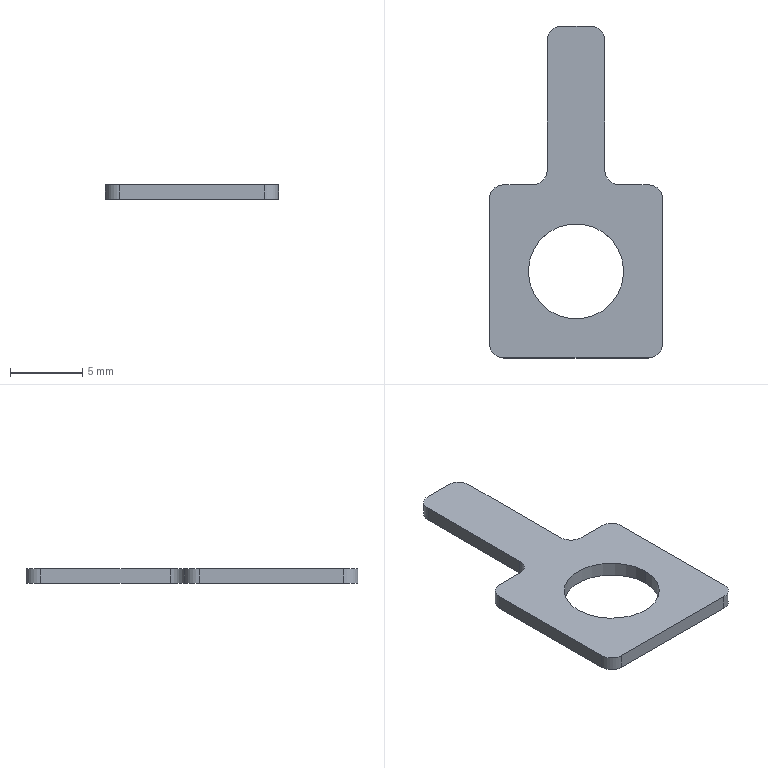Part | SolidWorks | features Extrusion 1, Fillet 1, HoleWzd 1 | 1 solid | 20 faces | box 12 x 23 x 1 mm | volume 152.93 mm3 | cylinder 10 | plane 10 | commonest cylinder face diameters 2 x8 6.6 x2
STEP:
#1=CARTESIAN_POINT('',(-3.3,0.,0.));
#2=VERTEX_POINT('',#1);
#3=CARTESIAN_POINT('',(3.3,0.,0.));
#4=VERTEX_POINT('',#3);
#5=CARTESIAN_POINT('',(0.,0.,0.));
#6=DIRECTION('',(0.,0.,1.));
#7=DIRECTION('',(1.,0.,0.));
#8=AXIS2_PLACEMENT_3D('',#5,#6,#7);
#9=CIRCLE('',#8,3.3);
#10=EDGE_CURVE('',#2,#4,#9,.T.);
#11=ORIENTED_EDGE('',*,*,#10,.F.);
#12=CARTESIAN_POINT('',(-3.3,0.,1.));
#13=VERTEX_POINT('',#12);
#14=CARTESIAN_POINT('',(-3.3,0.,1.));
#15=DIRECTION('',(0.,0.,1.));
#16=VECTOR('',#15,1000.);
#17=LINE('',#14,#16);
#18=EDGE_CURVE('',#2,#13,#17,.T.);
#19=ORIENTED_EDGE('',*,*,#18,.T.);
#20=CARTESIAN_POINT('',(3.3,0.,1.));
#21=VERTEX_POINT('',#20);
#22=CARTESIAN_POINT('',(0.,0.,1.));
#23=DIRECTION('',(0.,0.,1.));
#24=DIRECTION('',(1.,0.,0.));
#25=AXIS2_PLACEMENT_3D('',#22,#23,#24);
#26=CIRCLE('',#25,3.3);
#27=EDGE_CURVE('',#13,#21,#26,.T.);
#28=ORIENTED_EDGE('',*,*,#27,.T.);
#29=CARTESIAN_POINT('',(3.3,0.,1.));
#30=DIRECTION('',(0.,0.,1.));
#31=VECTOR('',#30,1000.);
#32=LINE('',#29,#31);
#33=EDGE_CURVE('',#4,#21,#32,.T.);
#34=ORIENTED_EDGE('',*,*,#33,.F.);
#35=EDGE_LOOP('',(#11,#19,#28,#34));
#36=FACE_OUTER_BOUND('',#35,.T.);
#37=CARTESIAN_POINT('',(0.,0.,1.));
#38=DIRECTION('',(0.,0.,1.));
#39=DIRECTION('',(1.,0.,0.));
#40=AXIS2_PLACEMENT_3D('',#37,#38,#39);
#41=CYLINDRICAL_SURFACE('',#40,3.3);
#42=ADVANCED_FACE('',(#36),#41,.F.);
#43=CARTESIAN_POINT('',(6.,-5.,1.));
#44=VERTEX_POINT('',#43);
#45=CARTESIAN_POINT('',(6.,5.,1.));
#46=VERTEX_POINT('',#45);
#47=CARTESIAN_POINT('',(6.,6.,1.));
#48=DIRECTION('',(0.,1.,0.));
#49=VECTOR('',#48,1000.);
#50=LINE('',#47,#49);
#51=EDGE_CURVE('',#44,#46,#50,.T.);
#52=ORIENTED_EDGE('',*,*,#51,.F.);
#53=CARTESIAN_POINT('',(6.,-5.,0.));
#54=VERTEX_POINT('',#53);
#55=CARTESIAN_POINT('',(6.,-5.,1.));
#56=DIRECTION('',(0.,0.,-1.));
#57=VECTOR('',#56,1000.);
#58=LINE('',#55,#57);
#59=EDGE_CURVE('',#44,#54,#58,.T.);
#60=ORIENTED_EDGE('',*,*,#59,.T.);
#61=CARTESIAN_POINT('',(6.,5.,0.));
#62=VERTEX_POINT('',#61);
#63=CARTESIAN_POINT('',(6.,6.,0.));
#64=DIRECTION('',(0.,1.,0.));
#65=VECTOR('',#64,1000.);
#66=LINE('',#63,#65);
#67=EDGE_CURVE('',#54,#62,#66,.T.);
#68=ORIENTED_EDGE('',*,*,#67,.T.);
#69=CARTESIAN_POINT('',(6.,5.,1.));
#70=DIRECTION('',(0.,0.,1.));
#71=VECTOR('',#70,1000.);
#72=LINE('',#69,#71);
#73=EDGE_CURVE('',#62,#46,#72,.T.);
#74=ORIENTED_EDGE('',*,*,#73,.T.);
#75=EDGE_LOOP('',(#52,#60,#68,#74));
#76=FACE_OUTER_BOUND('',#75,.T.);
#77=CARTESIAN_POINT('',(6.,6.,1.));
#78=DIRECTION('',(-1.,0.,0.));
#79=DIRECTION('',(0.,-1.,0.));
#80=AXIS2_PLACEMENT_3D('',#77,#78,#79);
#81=PLANE('',#80);
#82=ADVANCED_FACE('',(#76),#81,.F.);
#83=CARTESIAN_POINT('',(5.,6.,1.));
#84=VERTEX_POINT('',#83);
#85=CARTESIAN_POINT('',(3.,6.,1.));
#86=VERTEX_POINT('',#85);
#87=CARTESIAN_POINT('',(2.,6.,1.));
#88=DIRECTION('',(-1.,0.,0.));
#89=VECTOR('',#88,1000.);
#90=LINE('',#87,#89);
#91=EDGE_CURVE('',#84,#86,#90,.T.);
#92=ORIENTED_EDGE('',*,*,#91,.F.);
#93=CARTESIAN_POINT('',(5.,6.,0.));
#94=VERTEX_POINT('',#93);
#95=CARTESIAN_POINT('',(5.,6.,1.));
#96=DIRECTION('',(0.,0.,-1.));
#97=VECTOR('',#96,1000.);
#98=LINE('',#95,#97);
#99=EDGE_CURVE('',#84,#94,#98,.T.);
#100=ORIENTED_EDGE('',*,*,#99,.T.);
#101=CARTESIAN_POINT('',(3.,6.,0.));
#102=VERTEX_POINT('',#101);
#103=CARTESIAN_POINT('',(2.,6.,0.));
#104=DIRECTION('',(-1.,0.,0.));
#105=VECTOR('',#104,1000.);
#106=LINE('',#103,#105);
#107=EDGE_CURVE('',#94,#102,#106,.T.);
#108=ORIENTED_EDGE('',*,*,#107,.T.);
#109=CARTESIAN_POINT('',(3.,6.,1.));
#110=DIRECTION('',(0.,0.,1.));
#111=VECTOR('',#110,1000.);
#112=LINE('',#109,#111);
#113=EDGE_CURVE('',#102,#86,#112,.T.);
#114=ORIENTED_EDGE('',*,*,#113,.T.);
#115=EDGE_LOOP('',(#92,#100,#108,#114));
#116=FACE_OUTER_BOUND('',#115,.T.);
#117=CARTESIAN_POINT('',(2.,6.,1.));
#118=DIRECTION('',(0.,-1.,0.));
#119=DIRECTION('',(1.,0.,0.));
#120=AXIS2_PLACEMENT_3D('',#117,#118,#119);
#121=PLANE('',#120);
#122=ADVANCED_FACE('',(#116),#121,.F.);
#123=CARTESIAN_POINT('',(2.,7.,1.));
#124=VERTEX_POINT('',#123);
#125=CARTESIAN_POINT('',(2.,16.,1.));
#126=VERTEX_POINT('',#125);
#127=CARTESIAN_POINT('',(2.,6.,1.));
#128=DIRECTION('',(0.,1.,0.));
#129=VECTOR('',#128,1000.);
#130=LINE('',#127,#129);
#131=EDGE_CURVE('',#124,#126,#130,.T.);
#132=ORIENTED_EDGE('',*,*,#131,.F.);
#133=CARTESIAN_POINT('',(2.,7.,0.));
#134=VERTEX_POINT('',#133);
#135=CARTESIAN_POINT('',(2.,7.,0.));
#136=DIRECTION('',(0.,0.,-1.));
#137=VECTOR('',#136,1000.);
#138=LINE('',#135,#137);
#139=EDGE_CURVE('',#124,#134,#138,.T.);
#140=ORIENTED_EDGE('',*,*,#139,.T.);
#141=CARTESIAN_POINT('',(2.,16.,0.));
#142=VERTEX_POINT('',#141);
#143=CARTESIAN_POINT('',(2.,6.,0.));
#144=DIRECTION('',(0.,1.,0.));
#145=VECTOR('',#144,1000.);
#146=LINE('',#143,#145);
#147=EDGE_CURVE('',#134,#142,#146,.T.);
#148=ORIENTED_EDGE('',*,*,#147,.T.);
#149=CARTESIAN_POINT('',(2.,16.,1.));
#150=DIRECTION('',(0.,0.,1.));
#151=VECTOR('',#150,1000.);
#152=LINE('',#149,#151);
#153=EDGE_CURVE('',#142,#126,#152,.T.);
#154=ORIENTED_EDGE('',*,*,#153,.T.);
#155=EDGE_LOOP('',(#132,#140,#148,#154));
#156=FACE_OUTER_BOUND('',#155,.T.);
#157=CARTESIAN_POINT('',(2.,6.,1.));
#158=DIRECTION('',(-1.,0.,0.));
#159=DIRECTION('',(0.,-1.,0.));
#160=AXIS2_PLACEMENT_3D('',#157,#158,#159);
#161=PLANE('',#160);
#162=ADVANCED_FACE('',(#156),#161,.F.);
#163=CARTESIAN_POINT('',(1.,17.,0.));
#164=VERTEX_POINT('',#163);
#165=CARTESIAN_POINT('',(-1.,17.,0.));
#166=VERTEX_POINT('',#165);
#167=CARTESIAN_POINT('',(-2.,17.,0.));
#168=DIRECTION('',(-1.,0.,0.));
#169=VECTOR('',#168,1000.);
#170=LINE('',#167,#169);
#171=EDGE_CURVE('',#164,#166,#170,.T.);
#172=ORIENTED_EDGE('',*,*,#171,.T.);
#173=CARTESIAN_POINT('',(-1.,17.,1.));
#174=VERTEX_POINT('',#173);
#175=CARTESIAN_POINT('',(-1.,17.,1.));
#176=DIRECTION('',(0.,0.,1.));
#177=VECTOR('',#176,1000.);
#178=LINE('',#175,#177);
#179=EDGE_CURVE('',#166,#174,#178,.T.);
#180=ORIENTED_EDGE('',*,*,#179,.T.);
#181=CARTESIAN_POINT('',(1.,17.,1.));
#182=VERTEX_POINT('',#181);
#183=CARTESIAN_POINT('',(-2.,17.,1.));
#184=DIRECTION('',(-1.,0.,0.));
#185=VECTOR('',#184,1000.);
#186=LINE('',#183,#185);
#187=EDGE_CURVE('',#182,#174,#186,.T.);
#188=ORIENTED_EDGE('',*,*,#187,.F.);
#189=CARTESIAN_POINT('',(1.,17.,1.));
#190=DIRECTION('',(0.,0.,-1.));
#191=VECTOR('',#190,1000.);
#192=LINE('',#189,#191);
#193=EDGE_CURVE('',#182,#164,#192,.T.);
#194=ORIENTED_EDGE('',*,*,#193,.T.);
#195=EDGE_LOOP('',(#172,#180,#188,#194));
#196=FACE_OUTER_BOUND('',#195,.T.);
#197=CARTESIAN_POINT('',(-2.,17.,1.));
#198=DIRECTION('',(0.,-1.,0.));
#199=DIRECTION('',(0.,0.,-1.));
#200=AXIS2_PLACEMENT_3D('',#197,#198,#199);
#201=PLANE('',#200);
#202=ADVANCED_FACE('',(#196),#201,.F.);
#203=CARTESIAN_POINT('',(-2.,16.,0.));
#204=VERTEX_POINT('',#203);
#205=CARTESIAN_POINT('',(-2.,7.,0.));
#206=VERTEX_POINT('',#205);
#207=CARTESIAN_POINT('',(-2.,6.,0.));
#208=DIRECTION('',(0.,-1.,0.));
#209=VECTOR('',#208,1000.);
#210=LINE('',#207,#209);
#211=EDGE_CURVE('',#204,#206,#210,.T.);
#212=ORIENTED_EDGE('',*,*,#211,.T.);
#213=CARTESIAN_POINT('',(-2.,7.,1.));
#214=VERTEX_POINT('',#213);
#215=CARTESIAN_POINT('',(-2.,7.,1.));
#216=DIRECTION('',(0.,0.,1.));
#217=VECTOR('',#216,1000.);
#218=LINE('',#215,#217);
#219=EDGE_CURVE('',#206,#214,#218,.T.);
#220=ORIENTED_EDGE('',*,*,#219,.T.);
#221=CARTESIAN_POINT('',(-2.,16.,1.));
#222=VERTEX_POINT('',#221);
#223=CARTESIAN_POINT('',(-2.,6.,1.));
#224=DIRECTION('',(0.,-1.,0.));
#225=VECTOR('',#224,1000.);
#226=LINE('',#223,#225);
#227=EDGE_CURVE('',#222,#214,#226,.T.);
#228=ORIENTED_EDGE('',*,*,#227,.F.);
#229=CARTESIAN_POINT('',(-2.,16.,1.));
#230=DIRECTION('',(0.,0.,-1.));
#231=VECTOR('',#230,1000.);
#232=LINE('',#229,#231);
#233=EDGE_CURVE('',#222,#204,#232,.T.);
#234=ORIENTED_EDGE('',*,*,#233,.T.);
#235=EDGE_LOOP('',(#212,#220,#228,#234));
#236=FACE_OUTER_BOUND('',#235,.T.);
#237=CARTESIAN_POINT('',(-2.,6.,1.));
#238=DIRECTION('',(1.,0.,0.));
#239=DIRECTION('',(0.,0.,-1.));
#240=AXIS2_PLACEMENT_3D('',#237,#238,#239);
#241=PLANE('',#240);
#242=ADVANCED_FACE('',(#236),#241,.F.);
#243=CARTESIAN_POINT('',(-3.,6.,0.));
#244=VERTEX_POINT('',#243);
#245=CARTESIAN_POINT('',(-5.,6.,0.));
#246=VERTEX_POINT('',#245);
#247=CARTESIAN_POINT('',(-6.,6.,0.));
#248=DIRECTION('',(-1.,0.,0.));
#249=VECTOR('',#248,1000.);
#250=LINE('',#247,#249);
#251=EDGE_CURVE('',#244,#246,#250,.T.);
#252=ORIENTED_EDGE('',*,*,#251,.T.);
#253=CARTESIAN_POINT('',(-5.,6.,1.));
#254=VERTEX_POINT('',#253);
#255=CARTESIAN_POINT('',(-5.,6.,1.));
#256=DIRECTION('',(0.,0.,1.));
#257=VECTOR('',#256,1000.);
#258=LINE('',#255,#257);
#259=EDGE_CURVE('',#246,#254,#258,.T.);
#260=ORIENTED_EDGE('',*,*,#259,.T.);
#261=CARTESIAN_POINT('',(-3.,6.,1.));
#262=VERTEX_POINT('',#261);
#263=CARTESIAN_POINT('',(-6.,6.,1.));
#264=DIRECTION('',(-1.,0.,0.));
#265=VECTOR('',#264,1000.);
#266=LINE('',#263,#265);
#267=EDGE_CURVE('',#262,#254,#266,.T.);
#268=ORIENTED_EDGE('',*,*,#267,.F.);
#269=CARTESIAN_POINT('',(-3.,6.,0.));
#270=DIRECTION('',(0.,0.,-1.));
#271=VECTOR('',#270,1000.);
#272=LINE('',#269,#271);
#273=EDGE_CURVE('',#262,#244,#272,.T.);
#274=ORIENTED_EDGE('',*,*,#273,.T.);
#275=EDGE_LOOP('',(#252,#260,#268,#274));
#276=FACE_OUTER_BOUND('',#275,.T.);
#277=CARTESIAN_POINT('',(-6.,6.,1.));
#278=DIRECTION('',(0.,-1.,0.));
#279=DIRECTION('',(1.,0.,0.));
#280=AXIS2_PLACEMENT_3D('',#277,#278,#279);
#281=PLANE('',#280);
#282=ADVANCED_FACE('',(#276),#281,.F.);
#283=CARTESIAN_POINT('',(-6.,5.,1.));
#284=VERTEX_POINT('',#283);
#285=CARTESIAN_POINT('',(-6.,-5.,1.));
#286=VERTEX_POINT('',#285);
#287=CARTESIAN_POINT('',(-6.,6.,1.));
#288=DIRECTION('',(0.,-1.,0.));
#289=VECTOR('',#288,1000.);
#290=LINE('',#287,#289);
#291=EDGE_CURVE('',#284,#286,#290,.T.);
#292=ORIENTED_EDGE('',*,*,#291,.F.);
#293=CARTESIAN_POINT('',(-6.,5.,0.));
#294=VERTEX_POINT('',#293);
#295=CARTESIAN_POINT('',(-6.,5.,1.));
#296=DIRECTION('',(0.,0.,-1.));
#297=VECTOR('',#296,1000.);
#298=LINE('',#295,#297);
#299=EDGE_CURVE('',#284,#294,#298,.T.);
#300=ORIENTED_EDGE('',*,*,#299,.T.);
#301=CARTESIAN_POINT('',(-6.,-5.,0.));
#302=VERTEX_POINT('',#301);
#303=CARTESIAN_POINT('',(-6.,6.,0.));
#304=DIRECTION('',(0.,-1.,0.));
#305=VECTOR('',#304,1000.);
#306=LINE('',#303,#305);
#307=EDGE_CURVE('',#294,#302,#306,.T.);
#308=ORIENTED_EDGE('',*,*,#307,.T.);
#309=CARTESIAN_POINT('',(-6.,-5.,1.));
#310=DIRECTION('',(0.,0.,1.));
#311=VECTOR('',#310,1000.);
#312=LINE('',#309,#311);
#313=EDGE_CURVE('',#302,#286,#312,.T.);
#314=ORIENTED_EDGE('',*,*,#313,.T.);
#315=EDGE_LOOP('',(#292,#300,#308,#314));
#316=FACE_OUTER_BOUND('',#315,.T.);
#317=CARTESIAN_POINT('',(-6.,6.,1.));
#318=DIRECTION('',(1.,0.,0.));
#319=DIRECTION('',(0.,1.,0.));
#320=AXIS2_PLACEMENT_3D('',#317,#318,#319);
#321=PLANE('',#320);
#322=ADVANCED_FACE('',(#316),#321,.F.);
#323=CARTESIAN_POINT('',(-5.,-6.,1.));
#324=VERTEX_POINT('',#323);
#325=CARTESIAN_POINT('',(5.,-6.,1.));
#326=VERTEX_POINT('',#325);
#327=CARTESIAN_POINT('',(-6.,-6.,1.));
#328=DIRECTION('',(1.,0.,0.));
#329=VECTOR('',#328,1000.);
#330=LINE('',#327,#329);
#331=EDGE_CURVE('',#324,#326,#330,.T.);
#332=ORIENTED_EDGE('',*,*,#331,.F.);
#333=CARTESIAN_POINT('',(-5.,-6.,0.));
#334=VERTEX_POINT('',#333);
#335=CARTESIAN_POINT('',(-5.,-6.,1.));
#336=DIRECTION('',(0.,0.,-1.));
#337=VECTOR('',#336,1000.);
#338=LINE('',#335,#337);
#339=EDGE_CURVE('',#324,#334,#338,.T.);
#340=ORIENTED_EDGE('',*,*,#339,.T.);
#341=CARTESIAN_POINT('',(5.,-6.,0.));
#342=VERTEX_POINT('',#341);
#343=CARTESIAN_POINT('',(-6.,-6.,0.));
#344=DIRECTION('',(1.,0.,0.));
#345=VECTOR('',#344,1000.);
#346=LINE('',#343,#345);
#347=EDGE_CURVE('',#334,#342,#346,.T.);
#348=ORIENTED_EDGE('',*,*,#347,.T.);
#349=CARTESIAN_POINT('',(5.,-6.,1.));
#350=DIRECTION('',(0.,0.,1.));
#351=VECTOR('',#350,1000.);
#352=LINE('',#349,#351);
#353=EDGE_CURVE('',#342,#326,#352,.T.);
#354=ORIENTED_EDGE('',*,*,#353,.T.);
#355=EDGE_LOOP('',(#332,#340,#348,#354));
#356=FACE_OUTER_BOUND('',#355,.T.);
#357=CARTESIAN_POINT('',(-6.,-6.,1.));
#358=DIRECTION('',(0.,1.,0.));
#359=DIRECTION('',(0.,0.,1.));
#360=AXIS2_PLACEMENT_3D('',#357,#358,#359);
#361=PLANE('',#360);
#362=ADVANCED_FACE('',(#356),#361,.F.);
#363=CARTESIAN_POINT('',(0.,0.,1.));
#364=DIRECTION('',(0.,0.,1.));
#365=DIRECTION('',(1.,0.,0.));
#366=AXIS2_PLACEMENT_3D('',#363,#364,#365);
#367=CIRCLE('',#366,3.3);
#368=EDGE_CURVE('',#21,#13,#367,.T.);
#369=ORIENTED_EDGE('',*,*,#368,.F.);
#370=ORIENTED_EDGE('',*,*,#27,.F.);
#371=EDGE_LOOP('',(#369,#370));
#372=FACE_BOUND('',#371,.T.);
#373=ORIENTED_EDGE('',*,*,#267,.T.);
#374=CARTESIAN_POINT('',(-5.,5.,1.));
#375=DIRECTION('',(0.,0.,1.));
#376=DIRECTION('',(1.,0.,0.));
#377=AXIS2_PLACEMENT_3D('',#374,#375,#376);
#378=CIRCLE('',#377,1.);
#379=EDGE_CURVE('',#254,#284,#378,.T.);
#380=ORIENTED_EDGE('',*,*,#379,.T.);
#381=ORIENTED_EDGE('',*,*,#291,.T.);
#382=CARTESIAN_POINT('',(-5.,-5.,1.));
#383=DIRECTION('',(0.,0.,1.));
#384=DIRECTION('',(1.,0.,0.));
#385=AXIS2_PLACEMENT_3D('',#382,#383,#384);
#386=CIRCLE('',#385,1.);
#387=EDGE_CURVE('',#286,#324,#386,.T.);
#388=ORIENTED_EDGE('',*,*,#387,.T.);
#389=ORIENTED_EDGE('',*,*,#331,.T.);
#390=CARTESIAN_POINT('',(5.,-5.,1.));
#391=DIRECTION('',(0.,0.,1.));
#392=DIRECTION('',(1.,0.,0.));
#393=AXIS2_PLACEMENT_3D('',#390,#391,#392);
#394=CIRCLE('',#393,1.);
#395=EDGE_CURVE('',#326,#44,#394,.T.);
#396=ORIENTED_EDGE('',*,*,#395,.T.);
#397=ORIENTED_EDGE('',*,*,#51,.T.);
#398=CARTESIAN_POINT('',(5.,5.,1.));
#399=DIRECTION('',(0.,0.,1.));
#400=DIRECTION('',(1.,0.,0.));
#401=AXIS2_PLACEMENT_3D('',#398,#399,#400);
#402=CIRCLE('',#401,1.);
#403=EDGE_CURVE('',#46,#84,#402,.T.);
#404=ORIENTED_EDGE('',*,*,#403,.T.);
#405=ORIENTED_EDGE('',*,*,#91,.T.);
#406=CARTESIAN_POINT('',(3.,7.,1.));
#407=DIRECTION('',(0.,0.,-1.));
#408=DIRECTION('',(1.,0.,0.));
#409=AXIS2_PLACEMENT_3D('',#406,#407,#408);
#410=CIRCLE('',#409,1.);
#411=EDGE_CURVE('',#86,#124,#410,.T.);
#412=ORIENTED_EDGE('',*,*,#411,.T.);
#413=ORIENTED_EDGE('',*,*,#131,.T.);
#414=CARTESIAN_POINT('',(1.,16.,1.));
#415=DIRECTION('',(0.,0.,1.));
#416=DIRECTION('',(1.,0.,0.));
#417=AXIS2_PLACEMENT_3D('',#414,#415,#416);
#418=CIRCLE('',#417,1.);
#419=EDGE_CURVE('',#126,#182,#418,.T.);
#420=ORIENTED_EDGE('',*,*,#419,.T.);
#421=ORIENTED_EDGE('',*,*,#187,.T.);
#422=CARTESIAN_POINT('',(-1.,16.,1.));
#423=DIRECTION('',(0.,0.,1.));
#424=DIRECTION('',(1.,0.,0.));
#425=AXIS2_PLACEMENT_3D('',#422,#423,#424);
#426=CIRCLE('',#425,1.);
#427=EDGE_CURVE('',#174,#222,#426,.T.);
#428=ORIENTED_EDGE('',*,*,#427,.T.);
#429=ORIENTED_EDGE('',*,*,#227,.T.);
#430=CARTESIAN_POINT('',(-3.,7.,1.));
#431=DIRECTION('',(0.,0.,-1.));
#432=DIRECTION('',(1.,0.,0.));
#433=AXIS2_PLACEMENT_3D('',#430,#431,#432);
#434=CIRCLE('',#433,1.);
#435=EDGE_CURVE('',#214,#262,#434,.T.);
#436=ORIENTED_EDGE('',*,*,#435,.T.);
#437=EDGE_LOOP('',(#373,#380,#381,#388,#389,#396,#397,#404,#405,#412,#413,#420,#421,#428,#429,#436));
#438=FACE_OUTER_BOUND('',#437,.T.);
#439=CARTESIAN_POINT('',(0.,0.,1.));
#440=DIRECTION('',(0.,0.,1.));
#441=DIRECTION('',(1.,0.,0.));
#442=AXIS2_PLACEMENT_3D('',#439,#440,#441);
#443=PLANE('',#442);
#444=ADVANCED_FACE('',(#372,#438),#443,.T.);
#445=CARTESIAN_POINT('',(0.,0.,0.));
#446=DIRECTION('',(0.,0.,1.));
#447=DIRECTION('',(1.,0.,0.));
#448=AXIS2_PLACEMENT_3D('',#445,#446,#447);
#449=CIRCLE('',#448,3.3);
#450=EDGE_CURVE('',#4,#2,#449,.T.);
#451=ORIENTED_EDGE('',*,*,#450,.T.);
#452=ORIENTED_EDGE('',*,*,#10,.T.);
#453=EDGE_LOOP('',(#451,#452));
#454=FACE_BOUND('',#453,.T.);
#455=ORIENTED_EDGE('',*,*,#307,.F.);
#456=CARTESIAN_POINT('',(-5.,5.,0.));
#457=DIRECTION('',(0.,0.,-1.));
#458=DIRECTION('',(1.,0.,0.));
#459=AXIS2_PLACEMENT_3D('',#456,#457,#458);
#460=CIRCLE('',#459,1.);
#461=EDGE_CURVE('',#294,#246,#460,.T.);
#462=ORIENTED_EDGE('',*,*,#461,.T.);
#463=ORIENTED_EDGE('',*,*,#251,.F.);
#464=CARTESIAN_POINT('',(-3.,7.,0.));
#465=DIRECTION('',(0.,0.,1.));
#466=DIRECTION('',(1.,0.,0.));
#467=AXIS2_PLACEMENT_3D('',#464,#465,#466);
#468=CIRCLE('',#467,1.);
#469=EDGE_CURVE('',#244,#206,#468,.T.);
#470=ORIENTED_EDGE('',*,*,#469,.T.);
#471=ORIENTED_EDGE('',*,*,#211,.F.);
#472=CARTESIAN_POINT('',(-1.,16.,0.));
#473=DIRECTION('',(0.,0.,-1.));
#474=DIRECTION('',(1.,0.,0.));
#475=AXIS2_PLACEMENT_3D('',#472,#473,#474);
#476=CIRCLE('',#475,1.);
#477=EDGE_CURVE('',#204,#166,#476,.T.);
#478=ORIENTED_EDGE('',*,*,#477,.T.);
#479=ORIENTED_EDGE('',*,*,#171,.F.);
#480=CARTESIAN_POINT('',(1.,16.,0.));
#481=DIRECTION('',(0.,0.,-1.));
#482=DIRECTION('',(1.,0.,0.));
#483=AXIS2_PLACEMENT_3D('',#480,#481,#482);
#484=CIRCLE('',#483,1.);
#485=EDGE_CURVE('',#164,#142,#484,.T.);
#486=ORIENTED_EDGE('',*,*,#485,.T.);
#487=ORIENTED_EDGE('',*,*,#147,.F.);
#488=CARTESIAN_POINT('',(3.,7.,0.));
#489=DIRECTION('',(0.,0.,1.));
#490=DIRECTION('',(1.,0.,0.));
#491=AXIS2_PLACEMENT_3D('',#488,#489,#490);
#492=CIRCLE('',#491,1.);
#493=EDGE_CURVE('',#134,#102,#492,.T.);
#494=ORIENTED_EDGE('',*,*,#493,.T.);
#495=ORIENTED_EDGE('',*,*,#107,.F.);
#496=CARTESIAN_POINT('',(5.,5.,0.));
#497=DIRECTION('',(0.,0.,-1.));
#498=DIRECTION('',(1.,0.,0.));
#499=AXIS2_PLACEMENT_3D('',#496,#497,#498);
#500=CIRCLE('',#499,1.);
#501=EDGE_CURVE('',#94,#62,#500,.T.);
#502=ORIENTED_EDGE('',*,*,#501,.T.);
#503=ORIENTED_EDGE('',*,*,#67,.F.);
#504=CARTESIAN_POINT('',(5.,-5.,0.));
#505=DIRECTION('',(0.,0.,-1.));
#506=DIRECTION('',(1.,0.,0.));
#507=AXIS2_PLACEMENT_3D('',#504,#505,#506);
#508=CIRCLE('',#507,1.);
#509=EDGE_CURVE('',#54,#342,#508,.T.);
#510=ORIENTED_EDGE('',*,*,#509,.T.);
#511=ORIENTED_EDGE('',*,*,#347,.F.);
#512=CARTESIAN_POINT('',(-5.,-5.,0.));
#513=DIRECTION('',(0.,0.,-1.));
#514=DIRECTION('',(1.,0.,0.));
#515=AXIS2_PLACEMENT_3D('',#512,#513,#514);
#516=CIRCLE('',#515,1.);
#517=EDGE_CURVE('',#334,#302,#516,.T.);
#518=ORIENTED_EDGE('',*,*,#517,.T.);
#519=EDGE_LOOP('',(#455,#462,#463,#470,#471,#478,#479,#486,#487,#494,#495,#502,#503,#510,#511,#518));
#520=FACE_OUTER_BOUND('',#519,.T.);
#521=CARTESIAN_POINT('',(0.,0.,0.));
#522=DIRECTION('',(0.,0.,1.));
#523=DIRECTION('',(1.,0.,0.));
#524=AXIS2_PLACEMENT_3D('',#521,#522,#523);
#525=PLANE('',#524);
#526=ADVANCED_FACE('',(#454,#520),#525,.F.);
#527=ORIENTED_EDGE('',*,*,#18,.F.);
#528=ORIENTED_EDGE('',*,*,#450,.F.);
#529=ORIENTED_EDGE('',*,*,#33,.T.);
#530=ORIENTED_EDGE('',*,*,#368,.T.);
#531=EDGE_LOOP('',(#527,#528,#529,#530));
#532=FACE_OUTER_BOUND('',#531,.T.);
#533=CARTESIAN_POINT('',(0.,0.,1.));
#534=DIRECTION('',(0.,0.,1.));
#535=DIRECTION('',(1.,0.,0.));
#536=AXIS2_PLACEMENT_3D('',#533,#534,#535);
#537=CYLINDRICAL_SURFACE('',#536,3.3);
#538=ADVANCED_FACE('',(#532),#537,.F.);
#539=ORIENTED_EDGE('',*,*,#379,.F.);
#540=ORIENTED_EDGE('',*,*,#259,.F.);
#541=ORIENTED_EDGE('',*,*,#461,.F.);
#542=ORIENTED_EDGE('',*,*,#299,.F.);
#543=EDGE_LOOP('',(#539,#540,#541,#542));
#544=FACE_OUTER_BOUND('',#543,.T.);
#545=CARTESIAN_POINT('',(-5.,5.,1.));
#546=DIRECTION('',(0.,0.,-1.));
#547=DIRECTION('',(-1.,0.,0.));
#548=AXIS2_PLACEMENT_3D('',#545,#546,#547);
#549=CYLINDRICAL_SURFACE('',#548,1.);
#550=ADVANCED_FACE('',(#544),#549,.T.);
#551=ORIENTED_EDGE('',*,*,#387,.F.);
#552=ORIENTED_EDGE('',*,*,#313,.F.);
#553=ORIENTED_EDGE('',*,*,#517,.F.);
#554=ORIENTED_EDGE('',*,*,#339,.F.);
#555=EDGE_LOOP('',(#551,#552,#553,#554));
#556=FACE_OUTER_BOUND('',#555,.T.);
#557=CARTESIAN_POINT('',(-5.,-5.,1.));
#558=DIRECTION('',(0.,0.,-1.));
#559=DIRECTION('',(-1.,0.,0.));
#560=AXIS2_PLACEMENT_3D('',#557,#558,#559);
#561=CYLINDRICAL_SURFACE('',#560,1.);
#562=ADVANCED_FACE('',(#556),#561,.T.);
#563=ORIENTED_EDGE('',*,*,#395,.F.);
#564=ORIENTED_EDGE('',*,*,#353,.F.);
#565=ORIENTED_EDGE('',*,*,#509,.F.);
#566=ORIENTED_EDGE('',*,*,#59,.F.);
#567=EDGE_LOOP('',(#563,#564,#565,#566));
#568=FACE_OUTER_BOUND('',#567,.T.);
#569=CARTESIAN_POINT('',(5.,-5.,1.));
#570=DIRECTION('',(0.,0.,-1.));
#571=DIRECTION('',(-1.,0.,0.));
#572=AXIS2_PLACEMENT_3D('',#569,#570,#571);
#573=CYLINDRICAL_SURFACE('',#572,1.);
#574=ADVANCED_FACE('',(#568),#573,.T.);
#575=ORIENTED_EDGE('',*,*,#403,.F.);
#576=ORIENTED_EDGE('',*,*,#73,.F.);
#577=ORIENTED_EDGE('',*,*,#501,.F.);
#578=ORIENTED_EDGE('',*,*,#99,.F.);
#579=EDGE_LOOP('',(#575,#576,#577,#578));
#580=FACE_OUTER_BOUND('',#579,.T.);
#581=CARTESIAN_POINT('',(5.,5.,1.));
#582=DIRECTION('',(0.,0.,-1.));
#583=DIRECTION('',(-1.,0.,0.));
#584=AXIS2_PLACEMENT_3D('',#581,#582,#583);
#585=CYLINDRICAL_SURFACE('',#584,1.);
#586=ADVANCED_FACE('',(#580),#585,.T.);
#587=ORIENTED_EDGE('',*,*,#411,.F.);
#588=ORIENTED_EDGE('',*,*,#113,.F.);
#589=ORIENTED_EDGE('',*,*,#493,.F.);
#590=ORIENTED_EDGE('',*,*,#139,.F.);
#591=EDGE_LOOP('',(#587,#588,#589,#590));
#592=FACE_OUTER_BOUND('',#591,.T.);
#593=CARTESIAN_POINT('',(3.,7.,1.));
#594=DIRECTION('',(0.,0.,1.));
#595=DIRECTION('',(1.,0.,0.));
#596=AXIS2_PLACEMENT_3D('',#593,#594,#595);
#597=CYLINDRICAL_SURFACE('',#596,1.);
#598=ADVANCED_FACE('',(#592),#597,.F.);
#599=ORIENTED_EDGE('',*,*,#435,.F.);
#600=ORIENTED_EDGE('',*,*,#219,.F.);
#601=ORIENTED_EDGE('',*,*,#469,.F.);
#602=ORIENTED_EDGE('',*,*,#273,.F.);
#603=EDGE_LOOP('',(#599,#600,#601,#602));
#604=FACE_OUTER_BOUND('',#603,.T.);
#605=CARTESIAN_POINT('',(-3.,7.,1.));
#606=DIRECTION('',(0.,0.,1.));
#607=DIRECTION('',(1.,0.,0.));
#608=AXIS2_PLACEMENT_3D('',#605,#606,#607);
#609=CYLINDRICAL_SURFACE('',#608,1.);
#610=ADVANCED_FACE('',(#604),#609,.F.);
#611=ORIENTED_EDGE('',*,*,#427,.F.);
#612=ORIENTED_EDGE('',*,*,#179,.F.);
#613=ORIENTED_EDGE('',*,*,#477,.F.);
#614=ORIENTED_EDGE('',*,*,#233,.F.);
#615=EDGE_LOOP('',(#611,#612,#613,#614));
#616=FACE_OUTER_BOUND('',#615,.T.);
#617=CARTESIAN_POINT('',(-1.,16.,1.));
#618=DIRECTION('',(0.,0.,-1.));
#619=DIRECTION('',(-1.,0.,0.));
#620=AXIS2_PLACEMENT_3D('',#617,#618,#619);
#621=CYLINDRICAL_SURFACE('',#620,1.);
#622=ADVANCED_FACE('',(#616),#621,.T.);
#623=ORIENTED_EDGE('',*,*,#419,.F.);
#624=ORIENTED_EDGE('',*,*,#153,.F.);
#625=ORIENTED_EDGE('',*,*,#485,.F.);
#626=ORIENTED_EDGE('',*,*,#193,.F.);
#627=EDGE_LOOP('',(#623,#624,#625,#626));
#628=FACE_OUTER_BOUND('',#627,.T.);
#629=CARTESIAN_POINT('',(1.,16.,1.));
#630=DIRECTION('',(0.,0.,-1.));
#631=DIRECTION('',(-1.,0.,0.));
#632=AXIS2_PLACEMENT_3D('',#629,#630,#631);
#633=CYLINDRICAL_SURFACE('',#632,1.);
#634=ADVANCED_FACE('',(#628),#633,.T.);
#635=CLOSED_SHELL('',(#42,#82,#122,#162,#202,#242,#282,#322,#362,#444,#526,#538,#550,#562,#574,#586,#598,#610,#622,#634));
#636=MANIFOLD_SOLID_BREP('',#635);
#637=CARTESIAN_POINT('',(0.,0.,0.));
#638=DIRECTION('',(0.,0.,1.));
#639=DIRECTION('',(1.,0.,0.));
#640=AXIS2_PLACEMENT_3D('',#637,#638,#639);
#641=(LENGTH_UNIT()NAMED_UNIT(*)SI_UNIT(.MILLI.,.METRE.));
#642=UNCERTAINTY_MEASURE_WITH_UNIT(LENGTH_MEASURE(0.00001),#641,'','');
#643=(NAMED_UNIT(*)PLANE_ANGLE_UNIT()SI_UNIT($,.RADIAN.));
#644=(NAMED_UNIT(*)SI_UNIT($,.STERADIAN.)SOLID_ANGLE_UNIT());
#645=(GEOMETRIC_REPRESENTATION_CONTEXT(3)GLOBAL_UNCERTAINTY_ASSIGNED_CONTEXT((#642))GLOBAL_UNIT_ASSIGNED_CONTEXT((#641,#643,#644))REPRESENTATION_CONTEXT('',''));
#646=ADVANCED_BREP_SHAPE_REPRESENTATION('',(#636,#640),#645);